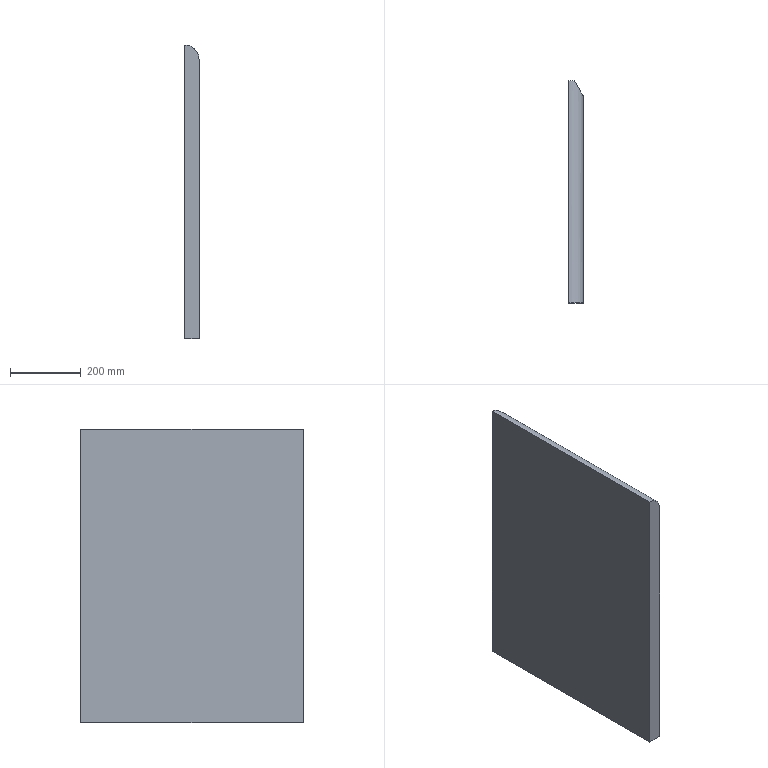Part | SolidWorks | features CutThin 1, Extrusion 1, Fillet 1 | 1 solid | 17 faces | box 40 x 630 x 832.5 mm | volume 20321060 mm3 | plane 16 | cylinder 1 | commonest cylinder face diameters 80 x1
STEP:
#1=CARTESIAN_POINT('',(0.,0.,832.5));
#2=VERTEX_POINT('',#1);
#3=CARTESIAN_POINT('',(0.,0.,0.));
#4=VERTEX_POINT('',#3);
#5=CARTESIAN_POINT('',(0.,0.,832.5));
#6=DIRECTION('',(0.,0.,-1.));
#7=VECTOR('',#6,1000.);
#8=LINE('',#5,#7);
#9=EDGE_CURVE('',#2,#4,#8,.T.);
#10=ORIENTED_EDGE('',*,*,#9,.F.);
#11=CARTESIAN_POINT('',(15.,0.,829.581));
#12=VERTEX_POINT('',#11);
#13=CARTESIAN_POINT('',(0.,0.,792.5));
#14=DIRECTION('',(0.,1.,0.));
#15=DIRECTION('',(0.,0.,-1.));
#16=AXIS2_PLACEMENT_3D('',#13,#14,#15);
#17=CIRCLE('',#16,40.);
#18=EDGE_CURVE('',#2,#12,#17,.T.);
#19=ORIENTED_EDGE('',*,*,#18,.T.);
#20=CARTESIAN_POINT('',(15.,0.,0.));
#21=VERTEX_POINT('',#20);
#22=CARTESIAN_POINT('',(15.,0.,832.5));
#23=DIRECTION('',(0.,0.,-1.));
#24=VECTOR('',#23,1000.);
#25=LINE('',#22,#24);
#26=EDGE_CURVE('',#12,#21,#25,.T.);
#27=ORIENTED_EDGE('',*,*,#26,.T.);
#28=CARTESIAN_POINT('',(0.,0.,0.));
#29=DIRECTION('',(-1.,0.,0.));
#30=VECTOR('',#29,1000.);
#31=LINE('',#28,#30);
#32=EDGE_CURVE('',#21,#4,#31,.T.);
#33=ORIENTED_EDGE('',*,*,#32,.T.);
#34=EDGE_LOOP('',(#10,#19,#27,#33));
#35=FACE_OUTER_BOUND('',#34,.T.);
#36=CARTESIAN_POINT('',(0.,0.,832.5));
#37=DIRECTION('',(0.,-1.,0.));
#38=DIRECTION('',(0.,0.,-1.));
#39=AXIS2_PLACEMENT_3D('',#36,#37,#38);
#40=PLANE('',#39);
#41=ADVANCED_FACE('',(#35),#40,.F.);
#42=CARTESIAN_POINT('',(0.,-630.,0.));
#43=VERTEX_POINT('',#42);
#44=CARTESIAN_POINT('',(0.,0.,0.));
#45=DIRECTION('',(0.,-1.,0.));
#46=VECTOR('',#45,1000.);
#47=LINE('',#44,#46);
#48=EDGE_CURVE('',#4,#43,#47,.T.);
#49=ORIENTED_EDGE('',*,*,#48,.T.);
#50=CARTESIAN_POINT('',(0.,-630.,832.5));
#51=VERTEX_POINT('',#50);
#52=CARTESIAN_POINT('',(0.,-630.,832.5));
#53=DIRECTION('',(0.,0.,-1.));
#54=VECTOR('',#53,1000.);
#55=LINE('',#52,#54);
#56=EDGE_CURVE('',#51,#43,#55,.T.);
#57=ORIENTED_EDGE('',*,*,#56,.F.);
#58=CARTESIAN_POINT('',(0.,0.,832.5));
#59=DIRECTION('',(0.,-1.,0.));
#60=VECTOR('',#59,1000.);
#61=LINE('',#58,#60);
#62=EDGE_CURVE('',#2,#51,#61,.T.);
#63=ORIENTED_EDGE('',*,*,#62,.F.);
#64=ORIENTED_EDGE('',*,*,#9,.T.);
#65=EDGE_LOOP('',(#49,#57,#63,#64));
#66=FACE_OUTER_BOUND('',#65,.T.);
#67=CARTESIAN_POINT('',(0.,0.,832.5));
#68=DIRECTION('',(1.,0.,0.));
#69=DIRECTION('',(0.,1.,0.));
#70=AXIS2_PLACEMENT_3D('',#67,#68,#69);
#71=PLANE('',#70);
#72=ADVANCED_FACE('',(#66),#71,.F.);
#73=CARTESIAN_POINT('',(40.,-630.,792.5));
#74=VERTEX_POINT('',#73);
#75=CARTESIAN_POINT('',(40.,-630.,0.));
#76=VERTEX_POINT('',#75);
#77=CARTESIAN_POINT('',(40.,-630.,832.5));
#78=DIRECTION('',(0.,0.,-1.));
#79=VECTOR('',#78,1000.);
#80=LINE('',#77,#79);
#81=EDGE_CURVE('',#74,#76,#80,.T.);
#82=ORIENTED_EDGE('',*,*,#81,.F.);
#83=CARTESIAN_POINT('',(0.,-630.,792.5));
#84=DIRECTION('',(0.,-1.,0.));
#85=DIRECTION('',(0.,0.,1.));
#86=AXIS2_PLACEMENT_3D('',#83,#84,#85);
#87=CIRCLE('',#86,40.);
#88=EDGE_CURVE('',#74,#51,#87,.T.);
#89=ORIENTED_EDGE('',*,*,#88,.T.);
#90=ORIENTED_EDGE('',*,*,#56,.T.);
#91=CARTESIAN_POINT('',(0.,-630.,0.));
#92=DIRECTION('',(1.,0.,0.));
#93=VECTOR('',#92,1000.);
#94=LINE('',#91,#93);
#95=EDGE_CURVE('',#43,#76,#94,.T.);
#96=ORIENTED_EDGE('',*,*,#95,.T.);
#97=EDGE_LOOP('',(#82,#89,#90,#96));
#98=FACE_OUTER_BOUND('',#97,.T.);
#99=CARTESIAN_POINT('',(0.,-630.,832.5));
#100=DIRECTION('',(0.,1.,0.));
#101=DIRECTION('',(0.,0.,1.));
#102=AXIS2_PLACEMENT_3D('',#99,#100,#101);
#103=PLANE('',#102);
#104=ADVANCED_FACE('',(#98),#103,.F.);
#105=CARTESIAN_POINT('',(40.,-144.501,465.45));
#106=VERTEX_POINT('',#105);
#107=CARTESIAN_POINT('',(40.,-144.501,367.05));
#108=VERTEX_POINT('',#107);
#109=CARTESIAN_POINT('',(40.,-144.501,464.25));
#110=DIRECTION('',(0.,0.,-1.));
#111=VECTOR('',#110,1000.);
#112=LINE('',#109,#111);
#113=EDGE_CURVE('',#106,#108,#112,.T.);
#114=ORIENTED_EDGE('',*,*,#113,.F.);
#115=CARTESIAN_POINT('',(40.,-102.101,465.45));
#116=VERTEX_POINT('',#115);
#117=CARTESIAN_POINT('',(40.,-103.301,465.45));
#118=DIRECTION('',(0.,-1.,0.));
#119=VECTOR('',#118,1000.);
#120=LINE('',#117,#119);
#121=EDGE_CURVE('',#116,#106,#120,.T.);
#122=ORIENTED_EDGE('',*,*,#121,.F.);
#123=CARTESIAN_POINT('',(40.,-102.101,367.05));
#124=VERTEX_POINT('',#123);
#125=CARTESIAN_POINT('',(40.,-102.101,464.25));
#126=DIRECTION('',(0.,0.,1.));
#127=VECTOR('',#126,1000.);
#128=LINE('',#125,#127);
#129=EDGE_CURVE('',#124,#116,#128,.T.);
#130=ORIENTED_EDGE('',*,*,#129,.F.);
#131=CARTESIAN_POINT('',(40.,-103.301,367.05));
#132=DIRECTION('',(0.,1.,0.));
#133=VECTOR('',#132,1000.);
#134=LINE('',#131,#133);
#135=EDGE_CURVE('',#108,#124,#134,.T.);
#136=ORIENTED_EDGE('',*,*,#135,.F.);
#137=EDGE_LOOP('',(#114,#122,#130,#136));
#138=FACE_BOUND('',#137,.T.);
#139=CARTESIAN_POINT('',(40.,-43.301,792.5));
#140=VERTEX_POINT('',#139);
#141=CARTESIAN_POINT('',(40.,-43.301,0.));
#142=VERTEX_POINT('',#141);
#143=CARTESIAN_POINT('',(40.,-43.301,832.5));
#144=DIRECTION('',(0.,0.,-1.));
#145=VECTOR('',#144,1000.);
#146=LINE('',#143,#145);
#147=EDGE_CURVE('',#140,#142,#146,.T.);
#148=ORIENTED_EDGE('',*,*,#147,.F.);
#149=CARTESIAN_POINT('',(40.,-630.,792.5));
#150=DIRECTION('',(0.,-1.,0.));
#151=VECTOR('',#150,1000.);
#152=LINE('',#149,#151);
#153=EDGE_CURVE('',#140,#74,#152,.T.);
#154=ORIENTED_EDGE('',*,*,#153,.T.);
#155=ORIENTED_EDGE('',*,*,#81,.T.);
#156=CARTESIAN_POINT('',(40.,-630.,0.));
#157=DIRECTION('',(0.,1.,0.));
#158=VECTOR('',#157,1000.);
#159=LINE('',#156,#158);
#160=EDGE_CURVE('',#76,#142,#159,.T.);
#161=ORIENTED_EDGE('',*,*,#160,.T.);
#162=EDGE_LOOP('',(#148,#154,#155,#161));
#163=FACE_OUTER_BOUND('',#162,.T.);
#164=CARTESIAN_POINT('',(40.,-630.,832.5));
#165=DIRECTION('',(-1.,0.,0.));
#166=DIRECTION('',(0.,-1.,0.));
#167=AXIS2_PLACEMENT_3D('',#164,#165,#166);
#168=PLANE('',#167);
#169=ADVANCED_FACE('',(#138,#163),#168,.F.);
#170=ORIENTED_EDGE('',*,*,#26,.F.);
#171=CARTESIAN_POINT('',(15.,0.,829.581));
#172=CARTESIAN_POINT('',(30.596,-27.012,823.272));
#173=CARTESIAN_POINT('',(40.,-43.301,809.323));
#174=CARTESIAN_POINT('',(40.,-43.301,792.5));
#175=(BOUNDED_CURVE()B_SPLINE_CURVE(3,(#171,#172,#173,#174),.UNSPECIFIED.,.F.,.F.)B_SPLINE_CURVE_WITH_KNOTS((4,4),(5.097,6.283),.UNSPECIFIED.)CURVE()GEOMETRIC_REPRESENTATION_ITEM()RATIONAL_B_SPLINE_CURVE((1.,0.8861,0.8861,1.))REPRESENTATION_ITEM(''));
#176=EDGE_CURVE('',#12,#140,#175,.T.);
#177=ORIENTED_EDGE('',*,*,#176,.T.);
#178=ORIENTED_EDGE('',*,*,#147,.T.);
#179=CARTESIAN_POINT('',(15.,0.,0.));
#180=DIRECTION('',(-0.5,0.866,0.));
#181=VECTOR('',#180,1000.);
#182=LINE('',#179,#181);
#183=EDGE_CURVE('',#142,#21,#182,.T.);
#184=ORIENTED_EDGE('',*,*,#183,.T.);
#185=EDGE_LOOP('',(#170,#177,#178,#184));
#186=FACE_OUTER_BOUND('',#185,.T.);
#187=CARTESIAN_POINT('',(15.,0.,832.5));
#188=DIRECTION('',(-0.866,-0.5,0.));
#189=DIRECTION('',(0.5,-0.866,0.));
#190=AXIS2_PLACEMENT_3D('',#187,#188,#189);
#191=PLANE('',#190);
#192=ADVANCED_FACE('',(#186),#191,.F.);
#193=ORIENTED_EDGE('',*,*,#32,.F.);
#194=ORIENTED_EDGE('',*,*,#183,.F.);
#195=ORIENTED_EDGE('',*,*,#160,.F.);
#196=ORIENTED_EDGE('',*,*,#95,.F.);
#197=ORIENTED_EDGE('',*,*,#48,.F.);
#198=EDGE_LOOP('',(#193,#194,#195,#196,#197));
#199=FACE_OUTER_BOUND('',#198,.T.);
#200=CARTESIAN_POINT('',(0.,0.,0.));
#201=DIRECTION('',(0.,0.,1.));
#202=DIRECTION('',(1.,0.,0.));
#203=AXIS2_PLACEMENT_3D('',#200,#201,#202);
#204=PLANE('',#203);
#205=ADVANCED_FACE('',(#199),#204,.F.);
#206=ORIENTED_EDGE('',*,*,#121,.T.);
#207=CARTESIAN_POINT('',(38.,-144.501,465.45));
#208=VERTEX_POINT('',#207);
#209=CARTESIAN_POINT('',(38.,-144.501,465.45));
#210=DIRECTION('',(1.,0.,0.));
#211=VECTOR('',#210,1000.);
#212=LINE('',#209,#211);
#213=EDGE_CURVE('',#208,#106,#212,.T.);
#214=ORIENTED_EDGE('',*,*,#213,.F.);
#215=CARTESIAN_POINT('',(38.,-102.101,465.45));
#216=VERTEX_POINT('',#215);
#217=CARTESIAN_POINT('',(38.,-103.301,465.45));
#218=DIRECTION('',(0.,-1.,0.));
#219=VECTOR('',#218,1000.);
#220=LINE('',#217,#219);
#221=EDGE_CURVE('',#216,#208,#220,.T.);
#222=ORIENTED_EDGE('',*,*,#221,.F.);
#223=CARTESIAN_POINT('',(38.,-102.101,465.45));
#224=DIRECTION('',(1.,0.,0.));
#225=VECTOR('',#224,1000.);
#226=LINE('',#223,#225);
#227=EDGE_CURVE('',#216,#116,#226,.T.);
#228=ORIENTED_EDGE('',*,*,#227,.T.);
#229=EDGE_LOOP('',(#206,#214,#222,#228));
#230=FACE_OUTER_BOUND('',#229,.T.);
#231=CARTESIAN_POINT('',(38.,-103.301,465.45));
#232=DIRECTION('',(0.,0.,1.));
#233=DIRECTION('',(1.,0.,0.));
#234=AXIS2_PLACEMENT_3D('',#231,#232,#233);
#235=PLANE('',#234);
#236=ADVANCED_FACE('',(#230),#235,.F.);
#237=ORIENTED_EDGE('',*,*,#129,.T.);
#238=ORIENTED_EDGE('',*,*,#227,.F.);
#239=CARTESIAN_POINT('',(38.,-102.101,367.05));
#240=VERTEX_POINT('',#239);
#241=CARTESIAN_POINT('',(38.,-102.101,464.25));
#242=DIRECTION('',(0.,0.,1.));
#243=VECTOR('',#242,1000.);
#244=LINE('',#241,#243);
#245=EDGE_CURVE('',#240,#216,#244,.T.);
#246=ORIENTED_EDGE('',*,*,#245,.F.);
#247=CARTESIAN_POINT('',(38.,-102.101,367.05));
#248=DIRECTION('',(1.,0.,0.));
#249=VECTOR('',#248,1000.);
#250=LINE('',#247,#249);
#251=EDGE_CURVE('',#240,#124,#250,.T.);
#252=ORIENTED_EDGE('',*,*,#251,.T.);
#253=EDGE_LOOP('',(#237,#238,#246,#252));
#254=FACE_OUTER_BOUND('',#253,.T.);
#255=CARTESIAN_POINT('',(38.,-102.101,464.25));
#256=DIRECTION('',(0.,1.,0.));
#257=DIRECTION('',(0.,0.,1.));
#258=AXIS2_PLACEMENT_3D('',#255,#256,#257);
#259=PLANE('',#258);
#260=ADVANCED_FACE('',(#254),#259,.F.);
#261=ORIENTED_EDGE('',*,*,#135,.T.);
#262=ORIENTED_EDGE('',*,*,#251,.F.);
#263=CARTESIAN_POINT('',(38.,-144.501,367.05));
#264=VERTEX_POINT('',#263);
#265=CARTESIAN_POINT('',(38.,-103.301,367.05));
#266=DIRECTION('',(0.,1.,0.));
#267=VECTOR('',#266,1000.);
#268=LINE('',#265,#267);
#269=EDGE_CURVE('',#264,#240,#268,.T.);
#270=ORIENTED_EDGE('',*,*,#269,.F.);
#271=CARTESIAN_POINT('',(38.,-144.501,367.05));
#272=DIRECTION('',(1.,0.,0.));
#273=VECTOR('',#272,1000.);
#274=LINE('',#271,#273);
#275=EDGE_CURVE('',#264,#108,#274,.T.);
#276=ORIENTED_EDGE('',*,*,#275,.T.);
#277=EDGE_LOOP('',(#261,#262,#270,#276));
#278=FACE_OUTER_BOUND('',#277,.T.);
#279=CARTESIAN_POINT('',(38.,-103.301,367.05));
#280=DIRECTION('',(0.,0.,-1.));
#281=DIRECTION('',(0.,1.,0.));
#282=AXIS2_PLACEMENT_3D('',#279,#280,#281);
#283=PLANE('',#282);
#284=ADVANCED_FACE('',(#278),#283,.F.);
#285=ORIENTED_EDGE('',*,*,#113,.T.);
#286=ORIENTED_EDGE('',*,*,#275,.F.);
#287=CARTESIAN_POINT('',(38.,-144.501,464.25));
#288=DIRECTION('',(0.,0.,-1.));
#289=VECTOR('',#288,1000.);
#290=LINE('',#287,#289);
#291=EDGE_CURVE('',#208,#264,#290,.T.);
#292=ORIENTED_EDGE('',*,*,#291,.F.);
#293=ORIENTED_EDGE('',*,*,#213,.T.);
#294=EDGE_LOOP('',(#285,#286,#292,#293));
#295=FACE_OUTER_BOUND('',#294,.T.);
#296=CARTESIAN_POINT('',(38.,-144.501,464.25));
#297=DIRECTION('',(0.,-1.,0.));
#298=DIRECTION('',(1.,0.,0.));
#299=AXIS2_PLACEMENT_3D('',#296,#297,#298);
#300=PLANE('',#299);
#301=ADVANCED_FACE('',(#295),#300,.F.);
#302=CARTESIAN_POINT('',(38.,-103.301,368.25));
#303=VERTEX_POINT('',#302);
#304=CARTESIAN_POINT('',(38.,-103.301,464.25));
#305=VERTEX_POINT('',#304);
#306=CARTESIAN_POINT('',(38.,-103.301,464.25));
#307=DIRECTION('',(0.,0.,1.));
#308=VECTOR('',#307,1000.);
#309=LINE('',#306,#308);
#310=EDGE_CURVE('',#303,#305,#309,.T.);
#311=ORIENTED_EDGE('',*,*,#310,.F.);
#312=CARTESIAN_POINT('',(38.,-143.301,368.25));
#313=VERTEX_POINT('',#312);
#314=CARTESIAN_POINT('',(38.,-103.301,368.25));
#315=DIRECTION('',(0.,1.,0.));
#316=VECTOR('',#315,1000.);
#317=LINE('',#314,#316);
#318=EDGE_CURVE('',#313,#303,#317,.T.);
#319=ORIENTED_EDGE('',*,*,#318,.F.);
#320=CARTESIAN_POINT('',(38.,-143.301,464.25));
#321=VERTEX_POINT('',#320);
#322=CARTESIAN_POINT('',(38.,-143.301,464.25));
#323=DIRECTION('',(0.,0.,-1.));
#324=VECTOR('',#323,1000.);
#325=LINE('',#322,#324);
#326=EDGE_CURVE('',#321,#313,#325,.T.);
#327=ORIENTED_EDGE('',*,*,#326,.F.);
#328=CARTESIAN_POINT('',(38.,-103.301,464.25));
#329=DIRECTION('',(0.,-1.,0.));
#330=VECTOR('',#329,1000.);
#331=LINE('',#328,#330);
#332=EDGE_CURVE('',#305,#321,#331,.T.);
#333=ORIENTED_EDGE('',*,*,#332,.F.);
#334=EDGE_LOOP('',(#311,#319,#327,#333));
#335=FACE_BOUND('',#334,.T.);
#336=ORIENTED_EDGE('',*,*,#221,.T.);
#337=ORIENTED_EDGE('',*,*,#291,.T.);
#338=ORIENTED_EDGE('',*,*,#269,.T.);
#339=ORIENTED_EDGE('',*,*,#245,.T.);
#340=EDGE_LOOP('',(#336,#337,#338,#339));
#341=FACE_OUTER_BOUND('',#340,.T.);
#342=CARTESIAN_POINT('',(38.,0.,0.));
#343=DIRECTION('',(1.,0.,0.));
#344=DIRECTION('',(0.,0.,-1.));
#345=AXIS2_PLACEMENT_3D('',#342,#343,#344);
#346=PLANE('',#345);
#347=ADVANCED_FACE('',(#335,#341),#346,.T.);
#348=CARTESIAN_POINT('',(40.,-103.301,464.25));
#349=VERTEX_POINT('',#348);
#350=CARTESIAN_POINT('',(40.,-143.301,464.25));
#351=VERTEX_POINT('',#350);
#352=CARTESIAN_POINT('',(40.,-103.301,464.25));
#353=DIRECTION('',(0.,-1.,0.));
#354=VECTOR('',#353,1000.);
#355=LINE('',#352,#354);
#356=EDGE_CURVE('',#349,#351,#355,.T.);
#357=ORIENTED_EDGE('',*,*,#356,.F.);
#358=CARTESIAN_POINT('',(38.,-103.301,464.25));
#359=DIRECTION('',(1.,0.,0.));
#360=VECTOR('',#359,1000.);
#361=LINE('',#358,#360);
#362=EDGE_CURVE('',#305,#349,#361,.T.);
#363=ORIENTED_EDGE('',*,*,#362,.F.);
#364=ORIENTED_EDGE('',*,*,#332,.T.);
#365=CARTESIAN_POINT('',(38.,-143.301,464.25));
#366=DIRECTION('',(1.,0.,0.));
#367=VECTOR('',#366,1000.);
#368=LINE('',#365,#367);
#369=EDGE_CURVE('',#321,#351,#368,.T.);
#370=ORIENTED_EDGE('',*,*,#369,.T.);
#371=EDGE_LOOP('',(#357,#363,#364,#370));
#372=FACE_OUTER_BOUND('',#371,.T.);
#373=CARTESIAN_POINT('',(38.,-103.301,464.25));
#374=DIRECTION('',(0.,0.,1.));
#375=DIRECTION('',(1.,0.,0.));
#376=AXIS2_PLACEMENT_3D('',#373,#374,#375);
#377=PLANE('',#376);
#378=ADVANCED_FACE('',(#372),#377,.T.);
#379=CARTESIAN_POINT('',(40.,-103.301,368.25));
#380=VERTEX_POINT('',#379);
#381=CARTESIAN_POINT('',(40.,-103.301,464.25));
#382=DIRECTION('',(0.,0.,1.));
#383=VECTOR('',#382,1000.);
#384=LINE('',#381,#383);
#385=EDGE_CURVE('',#380,#349,#384,.T.);
#386=ORIENTED_EDGE('',*,*,#385,.F.);
#387=CARTESIAN_POINT('',(38.,-103.301,368.25));
#388=DIRECTION('',(1.,0.,0.));
#389=VECTOR('',#388,1000.);
#390=LINE('',#387,#389);
#391=EDGE_CURVE('',#303,#380,#390,.T.);
#392=ORIENTED_EDGE('',*,*,#391,.F.);
#393=ORIENTED_EDGE('',*,*,#310,.T.);
#394=ORIENTED_EDGE('',*,*,#362,.T.);
#395=EDGE_LOOP('',(#386,#392,#393,#394));
#396=FACE_OUTER_BOUND('',#395,.T.);
#397=CARTESIAN_POINT('',(38.,-103.301,464.25));
#398=DIRECTION('',(0.,1.,0.));
#399=DIRECTION('',(0.,0.,1.));
#400=AXIS2_PLACEMENT_3D('',#397,#398,#399);
#401=PLANE('',#400);
#402=ADVANCED_FACE('',(#396),#401,.T.);
#403=CARTESIAN_POINT('',(40.,-143.301,368.25));
#404=VERTEX_POINT('',#403);
#405=CARTESIAN_POINT('',(40.,-103.301,368.25));
#406=DIRECTION('',(0.,1.,0.));
#407=VECTOR('',#406,1000.);
#408=LINE('',#405,#407);
#409=EDGE_CURVE('',#404,#380,#408,.T.);
#410=ORIENTED_EDGE('',*,*,#409,.F.);
#411=CARTESIAN_POINT('',(38.,-143.301,368.25));
#412=DIRECTION('',(1.,0.,0.));
#413=VECTOR('',#412,1000.);
#414=LINE('',#411,#413);
#415=EDGE_CURVE('',#313,#404,#414,.T.);
#416=ORIENTED_EDGE('',*,*,#415,.F.);
#417=ORIENTED_EDGE('',*,*,#318,.T.);
#418=ORIENTED_EDGE('',*,*,#391,.T.);
#419=EDGE_LOOP('',(#410,#416,#417,#418));
#420=FACE_OUTER_BOUND('',#419,.T.);
#421=CARTESIAN_POINT('',(38.,-103.301,368.25));
#422=DIRECTION('',(0.,0.,-1.));
#423=DIRECTION('',(0.,1.,0.));
#424=AXIS2_PLACEMENT_3D('',#421,#422,#423);
#425=PLANE('',#424);
#426=ADVANCED_FACE('',(#420),#425,.T.);
#427=CARTESIAN_POINT('',(40.,-143.301,464.25));
#428=DIRECTION('',(0.,0.,-1.));
#429=VECTOR('',#428,1000.);
#430=LINE('',#427,#429);
#431=EDGE_CURVE('',#351,#404,#430,.T.);
#432=ORIENTED_EDGE('',*,*,#431,.F.);
#433=ORIENTED_EDGE('',*,*,#369,.F.);
#434=ORIENTED_EDGE('',*,*,#326,.T.);
#435=ORIENTED_EDGE('',*,*,#415,.T.);
#436=EDGE_LOOP('',(#432,#433,#434,#435));
#437=FACE_OUTER_BOUND('',#436,.T.);
#438=CARTESIAN_POINT('',(38.,-143.301,464.25));
#439=DIRECTION('',(0.,-1.,0.));
#440=DIRECTION('',(1.,0.,0.));
#441=AXIS2_PLACEMENT_3D('',#438,#439,#440);
#442=PLANE('',#441);
#443=ADVANCED_FACE('',(#437),#442,.T.);
#444=ORIENTED_EDGE('',*,*,#356,.T.);
#445=ORIENTED_EDGE('',*,*,#431,.T.);
#446=ORIENTED_EDGE('',*,*,#409,.T.);
#447=ORIENTED_EDGE('',*,*,#385,.T.);
#448=EDGE_LOOP('',(#444,#445,#446,#447));
#449=FACE_OUTER_BOUND('',#448,.T.);
#450=CARTESIAN_POINT('',(40.,-630.,832.5));
#451=DIRECTION('',(-1.,0.,0.));
#452=DIRECTION('',(0.,-1.,0.));
#453=AXIS2_PLACEMENT_3D('',#450,#451,#452);
#454=PLANE('',#453);
#455=ADVANCED_FACE('',(#449),#454,.F.);
#456=ORIENTED_EDGE('',*,*,#88,.F.);
#457=ORIENTED_EDGE('',*,*,#153,.F.);
#458=ORIENTED_EDGE('',*,*,#176,.F.);
#459=ORIENTED_EDGE('',*,*,#18,.F.);
#460=ORIENTED_EDGE('',*,*,#62,.T.);
#461=EDGE_LOOP('',(#456,#457,#458,#459,#460));
#462=FACE_OUTER_BOUND('',#461,.T.);
#463=CARTESIAN_POINT('',(0.,0.,792.5));
#464=DIRECTION('',(0.,-1.,0.));
#465=DIRECTION('',(1.,0.,0.));
#466=AXIS2_PLACEMENT_3D('',#463,#464,#465);
#467=CYLINDRICAL_SURFACE('',#466,40.);
#468=ADVANCED_FACE('',(#462),#467,.T.);
#469=CLOSED_SHELL('',(#41,#72,#104,#169,#192,#205,#236,#260,#284,#301,#347,#378,#402,#426,#443,#455,#468));
#470=MANIFOLD_SOLID_BREP('',#469);
#471=CARTESIAN_POINT('',(0.,0.,0.));
#472=DIRECTION('',(0.,0.,1.));
#473=DIRECTION('',(1.,0.,0.));
#474=AXIS2_PLACEMENT_3D('',#471,#472,#473);
#475=(LENGTH_UNIT()NAMED_UNIT(*)SI_UNIT(.MILLI.,.METRE.));
#476=UNCERTAINTY_MEASURE_WITH_UNIT(LENGTH_MEASURE(0.00001),#475,'','');
#477=(NAMED_UNIT(*)PLANE_ANGLE_UNIT()SI_UNIT($,.RADIAN.));
#478=(NAMED_UNIT(*)SI_UNIT($,.STERADIAN.)SOLID_ANGLE_UNIT());
#479=(GEOMETRIC_REPRESENTATION_CONTEXT(3)GLOBAL_UNCERTAINTY_ASSIGNED_CONTEXT((#476))GLOBAL_UNIT_ASSIGNED_CONTEXT((#475,#477,#478))REPRESENTATION_CONTEXT('',''));
#480=ADVANCED_BREP_SHAPE_REPRESENTATION('',(#470,#474),#479);